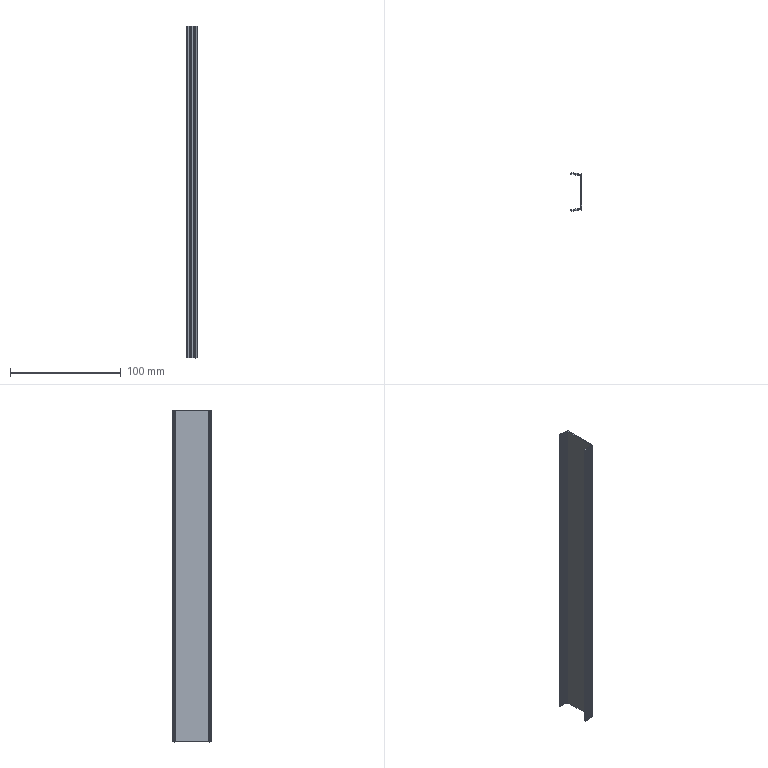Part | STEP file | slide rail 300-2 | 1 solid | 62 faces | box 10.373 x 34.385 x 300 mm | volume 15280 mm3 | plane 56 | cylinder 6 | commonest cylinder face diameters 0.4 x4 1 x2